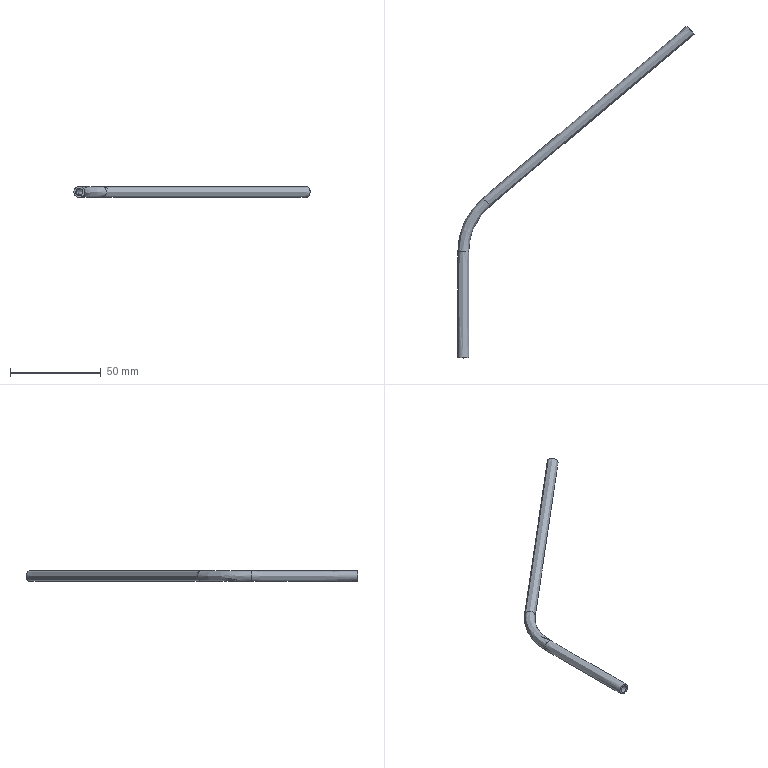Part | NX | features solid 2 | 1 solid | 8 faces | box 130.19 x 182.986 x 6 mm | volume 3719 mm3 | spline 6 | plane 2